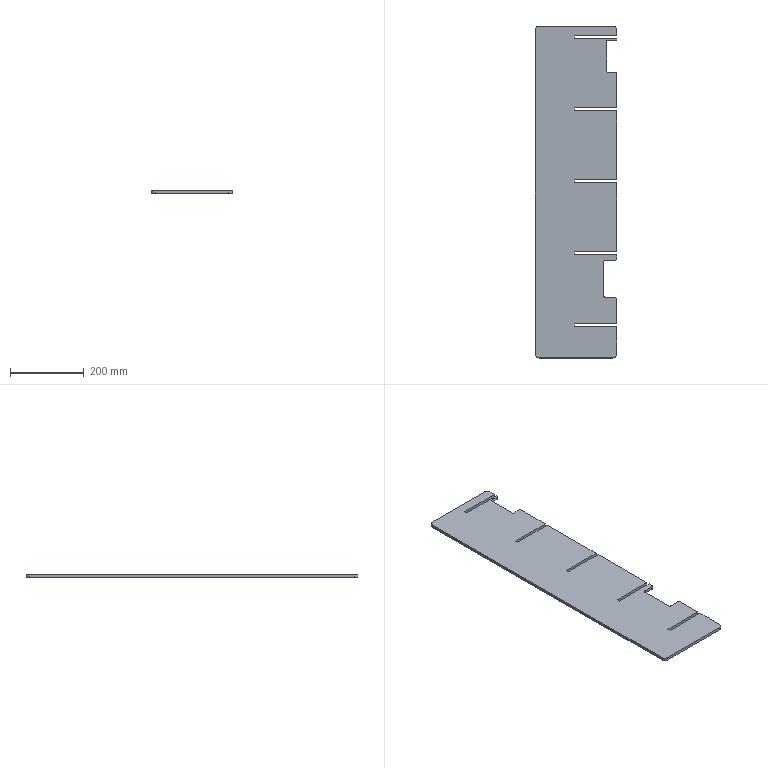Part | SolidWorks | features FlatPattern 1, SMBaseFlange 1, SheetMetal 1 | 1 solid | 46 faces | box 220 x 900 x 8 mm | volume 1500106 mm3 | plane 34 | cylinder 12 | commonest cylinder face diameters 4 x4 10 x4 20 x4
STEP:
#1=CARTESIAN_POINT('',(-1005.006,-530.938,0.));
#2=VERTEX_POINT('',#1);
#3=CARTESIAN_POINT('',(-995.006,-520.938,0.));
#4=VERTEX_POINT('',#3);
#5=CARTESIAN_POINT('',(-1005.006,-520.938,0.));
#6=DIRECTION('',(0.,0.,1.));
#7=DIRECTION('',(-1.,0.,0.));
#8=AXIS2_PLACEMENT_3D('',#5,#6,#7);
#9=CIRCLE('',#8,10.);
#10=EDGE_CURVE('',#2,#4,#9,.T.);
#11=ORIENTED_EDGE('',*,*,#10,.F.);
#12=CARTESIAN_POINT('',(-1005.006,-530.938,-8.));
#13=VERTEX_POINT('',#12);
#14=CARTESIAN_POINT('',(-1005.006,-530.938,-8.));
#15=DIRECTION('',(0.,0.,1.));
#16=VECTOR('',#15,1000.);
#17=LINE('',#14,#16);
#18=EDGE_CURVE('',#13,#2,#17,.T.);
#19=ORIENTED_EDGE('',*,*,#18,.F.);
#20=CARTESIAN_POINT('',(-995.006,-520.938,-8.));
#21=VERTEX_POINT('',#20);
#22=CARTESIAN_POINT('',(-1005.006,-520.938,-8.));
#23=DIRECTION('',(0.,0.,1.));
#24=DIRECTION('',(-1.,0.,0.));
#25=AXIS2_PLACEMENT_3D('',#22,#23,#24);
#26=CIRCLE('',#25,10.);
#27=EDGE_CURVE('',#13,#21,#26,.T.);
#28=ORIENTED_EDGE('',*,*,#27,.T.);
#29=CARTESIAN_POINT('',(-995.006,-520.938,-8.));
#30=DIRECTION('',(0.,0.,1.));
#31=VECTOR('',#30,1000.);
#32=LINE('',#29,#31);
#33=EDGE_CURVE('',#21,#4,#32,.T.);
#34=ORIENTED_EDGE('',*,*,#33,.T.);
#35=EDGE_LOOP('',(#11,#19,#28,#34));
#36=FACE_OUTER_BOUND('',#35,.T.);
#37=CARTESIAN_POINT('',(-1005.006,-520.938,-8.));
#38=DIRECTION('',(0.,0.,1.));
#39=DIRECTION('',(1.,0.,0.));
#40=AXIS2_PLACEMENT_3D('',#37,#38,#39);
#41=CYLINDRICAL_SURFACE('',#40,10.);
#42=ADVANCED_FACE('',(#36),#41,.T.);
#43=CARTESIAN_POINT('',(-1205.006,-530.938,0.));
#44=VERTEX_POINT('',#43);
#45=CARTESIAN_POINT('',(-1005.006,-530.938,0.));
#46=DIRECTION('',(1.,0.,0.));
#47=VECTOR('',#46,1000.);
#48=LINE('',#45,#47);
#49=EDGE_CURVE('',#44,#2,#48,.T.);
#50=ORIENTED_EDGE('',*,*,#49,.F.);
#51=CARTESIAN_POINT('',(-1205.006,-530.938,-8.));
#52=VERTEX_POINT('',#51);
#53=CARTESIAN_POINT('',(-1205.006,-530.938,-8.));
#54=DIRECTION('',(0.,0.,1.));
#55=VECTOR('',#54,1000.);
#56=LINE('',#53,#55);
#57=EDGE_CURVE('',#52,#44,#56,.T.);
#58=ORIENTED_EDGE('',*,*,#57,.F.);
#59=CARTESIAN_POINT('',(-1005.006,-530.938,-8.));
#60=DIRECTION('',(1.,0.,0.));
#61=VECTOR('',#60,1000.);
#62=LINE('',#59,#61);
#63=EDGE_CURVE('',#52,#13,#62,.T.);
#64=ORIENTED_EDGE('',*,*,#63,.T.);
#65=ORIENTED_EDGE('',*,*,#18,.T.);
#66=EDGE_LOOP('',(#50,#58,#64,#65));
#67=FACE_OUTER_BOUND('',#66,.T.);
#68=CARTESIAN_POINT('',(-1005.006,-530.938,-8.));
#69=DIRECTION('',(0.,-1.,0.));
#70=DIRECTION('',(1.,0.,0.));
#71=AXIS2_PLACEMENT_3D('',#68,#69,#70);
#72=PLANE('',#71);
#73=ADVANCED_FACE('',(#67),#72,.T.);
#74=CARTESIAN_POINT('',(-1215.006,-520.938,0.));
#75=VERTEX_POINT('',#74);
#76=CARTESIAN_POINT('',(-1205.006,-520.938,0.));
#77=DIRECTION('',(0.,0.,1.));
#78=DIRECTION('',(-1.,0.,0.));
#79=AXIS2_PLACEMENT_3D('',#76,#77,#78);
#80=CIRCLE('',#79,10.);
#81=EDGE_CURVE('',#75,#44,#80,.T.);
#82=ORIENTED_EDGE('',*,*,#81,.F.);
#83=CARTESIAN_POINT('',(-1215.006,-520.938,-8.));
#84=VERTEX_POINT('',#83);
#85=CARTESIAN_POINT('',(-1215.006,-520.938,-8.));
#86=DIRECTION('',(0.,0.,1.));
#87=VECTOR('',#86,1000.);
#88=LINE('',#85,#87);
#89=EDGE_CURVE('',#84,#75,#88,.T.);
#90=ORIENTED_EDGE('',*,*,#89,.F.);
#91=CARTESIAN_POINT('',(-1205.006,-520.938,-8.));
#92=DIRECTION('',(0.,0.,1.));
#93=DIRECTION('',(-1.,0.,0.));
#94=AXIS2_PLACEMENT_3D('',#91,#92,#93);
#95=CIRCLE('',#94,10.);
#96=EDGE_CURVE('',#84,#52,#95,.T.);
#97=ORIENTED_EDGE('',*,*,#96,.T.);
#98=ORIENTED_EDGE('',*,*,#57,.T.);
#99=EDGE_LOOP('',(#82,#90,#97,#98));
#100=FACE_OUTER_BOUND('',#99,.T.);
#101=CARTESIAN_POINT('',(-1205.006,-520.938,-8.));
#102=DIRECTION('',(0.,0.,1.));
#103=DIRECTION('',(1.,0.,0.));
#104=AXIS2_PLACEMENT_3D('',#101,#102,#103);
#105=CYLINDRICAL_SURFACE('',#104,10.);
#106=ADVANCED_FACE('',(#100),#105,.T.);
#107=CARTESIAN_POINT('',(-1215.006,359.062,0.));
#108=VERTEX_POINT('',#107);
#109=CARTESIAN_POINT('',(-1215.006,359.062,0.));
#110=DIRECTION('',(0.,-1.,0.));
#111=VECTOR('',#110,1000.);
#112=LINE('',#109,#111);
#113=EDGE_CURVE('',#108,#75,#112,.T.);
#114=ORIENTED_EDGE('',*,*,#113,.F.);
#115=CARTESIAN_POINT('',(-1215.006,359.062,-8.));
#116=VERTEX_POINT('',#115);
#117=CARTESIAN_POINT('',(-1215.006,359.062,-8.));
#118=DIRECTION('',(0.,0.,1.));
#119=VECTOR('',#118,1000.);
#120=LINE('',#117,#119);
#121=EDGE_CURVE('',#116,#108,#120,.T.);
#122=ORIENTED_EDGE('',*,*,#121,.F.);
#123=CARTESIAN_POINT('',(-1215.006,359.062,-8.));
#124=DIRECTION('',(0.,-1.,0.));
#125=VECTOR('',#124,1000.);
#126=LINE('',#123,#125);
#127=EDGE_CURVE('',#116,#84,#126,.T.);
#128=ORIENTED_EDGE('',*,*,#127,.T.);
#129=ORIENTED_EDGE('',*,*,#89,.T.);
#130=EDGE_LOOP('',(#114,#122,#128,#129));
#131=FACE_OUTER_BOUND('',#130,.T.);
#132=CARTESIAN_POINT('',(-1215.006,359.062,-8.));
#133=DIRECTION('',(-1.,0.,0.));
#134=DIRECTION('',(0.,0.,1.));
#135=AXIS2_PLACEMENT_3D('',#132,#133,#134);
#136=PLANE('',#135);
#137=ADVANCED_FACE('',(#131),#136,.T.);
#138=CARTESIAN_POINT('',(-1205.006,369.062,0.));
#139=VERTEX_POINT('',#138);
#140=CARTESIAN_POINT('',(-1205.006,359.062,0.));
#141=DIRECTION('',(0.,0.,1.));
#142=DIRECTION('',(1.,0.,0.));
#143=AXIS2_PLACEMENT_3D('',#140,#141,#142);
#144=CIRCLE('',#143,10.);
#145=EDGE_CURVE('',#139,#108,#144,.T.);
#146=ORIENTED_EDGE('',*,*,#145,.F.);
#147=CARTESIAN_POINT('',(-1205.006,369.062,-8.));
#148=VERTEX_POINT('',#147);
#149=CARTESIAN_POINT('',(-1205.006,369.062,-8.));
#150=DIRECTION('',(0.,0.,1.));
#151=VECTOR('',#150,1000.);
#152=LINE('',#149,#151);
#153=EDGE_CURVE('',#148,#139,#152,.T.);
#154=ORIENTED_EDGE('',*,*,#153,.F.);
#155=CARTESIAN_POINT('',(-1205.006,359.062,-8.));
#156=DIRECTION('',(0.,0.,1.));
#157=DIRECTION('',(1.,0.,0.));
#158=AXIS2_PLACEMENT_3D('',#155,#156,#157);
#159=CIRCLE('',#158,10.);
#160=EDGE_CURVE('',#148,#116,#159,.T.);
#161=ORIENTED_EDGE('',*,*,#160,.T.);
#162=ORIENTED_EDGE('',*,*,#121,.T.);
#163=EDGE_LOOP('',(#146,#154,#161,#162));
#164=FACE_OUTER_BOUND('',#163,.T.);
#165=CARTESIAN_POINT('',(-1205.006,359.062,-8.));
#166=DIRECTION('',(0.,0.,1.));
#167=DIRECTION('',(1.,0.,0.));
#168=AXIS2_PLACEMENT_3D('',#165,#166,#167);
#169=CYLINDRICAL_SURFACE('',#168,10.);
#170=ADVANCED_FACE('',(#164),#169,.T.);
#171=CARTESIAN_POINT('',(-1005.006,369.062,0.));
#172=VERTEX_POINT('',#171);
#173=CARTESIAN_POINT('',(-1005.006,369.062,0.));
#174=DIRECTION('',(-1.,0.,0.));
#175=VECTOR('',#174,1000.);
#176=LINE('',#173,#175);
#177=EDGE_CURVE('',#172,#139,#176,.T.);
#178=ORIENTED_EDGE('',*,*,#177,.F.);
#179=CARTESIAN_POINT('',(-1005.006,369.062,-8.));
#180=VERTEX_POINT('',#179);
#181=CARTESIAN_POINT('',(-1005.006,369.062,-8.));
#182=DIRECTION('',(0.,0.,1.));
#183=VECTOR('',#182,1000.);
#184=LINE('',#181,#183);
#185=EDGE_CURVE('',#180,#172,#184,.T.);
#186=ORIENTED_EDGE('',*,*,#185,.F.);
#187=CARTESIAN_POINT('',(-1005.006,369.062,-8.));
#188=DIRECTION('',(-1.,0.,0.));
#189=VECTOR('',#188,1000.);
#190=LINE('',#187,#189);
#191=EDGE_CURVE('',#180,#148,#190,.T.);
#192=ORIENTED_EDGE('',*,*,#191,.T.);
#193=ORIENTED_EDGE('',*,*,#153,.T.);
#194=EDGE_LOOP('',(#178,#186,#192,#193));
#195=FACE_OUTER_BOUND('',#194,.T.);
#196=CARTESIAN_POINT('',(-1005.006,369.062,-8.));
#197=DIRECTION('',(0.,1.,0.));
#198=DIRECTION('',(0.,0.,1.));
#199=AXIS2_PLACEMENT_3D('',#196,#197,#198);
#200=PLANE('',#199);
#201=ADVANCED_FACE('',(#195),#200,.T.);
#202=CARTESIAN_POINT('',(-995.006,359.062,0.));
#203=VERTEX_POINT('',#202);
#204=CARTESIAN_POINT('',(-1005.006,359.062,0.));
#205=DIRECTION('',(0.,0.,1.));
#206=DIRECTION('',(-1.,0.,0.));
#207=AXIS2_PLACEMENT_3D('',#204,#205,#206);
#208=CIRCLE('',#207,10.);
#209=EDGE_CURVE('',#203,#172,#208,.T.);
#210=ORIENTED_EDGE('',*,*,#209,.F.);
#211=CARTESIAN_POINT('',(-995.006,359.062,-8.));
#212=VERTEX_POINT('',#211);
#213=CARTESIAN_POINT('',(-995.006,359.062,-8.));
#214=DIRECTION('',(0.,0.,1.));
#215=VECTOR('',#214,1000.);
#216=LINE('',#213,#215);
#217=EDGE_CURVE('',#212,#203,#216,.T.);
#218=ORIENTED_EDGE('',*,*,#217,.F.);
#219=CARTESIAN_POINT('',(-1005.006,359.062,-8.));
#220=DIRECTION('',(0.,0.,1.));
#221=DIRECTION('',(-1.,0.,0.));
#222=AXIS2_PLACEMENT_3D('',#219,#220,#221);
#223=CIRCLE('',#222,10.);
#224=EDGE_CURVE('',#212,#180,#223,.T.);
#225=ORIENTED_EDGE('',*,*,#224,.T.);
#226=ORIENTED_EDGE('',*,*,#185,.T.);
#227=EDGE_LOOP('',(#210,#218,#225,#226));
#228=FACE_OUTER_BOUND('',#227,.T.);
#229=CARTESIAN_POINT('',(-1005.006,359.062,-8.));
#230=DIRECTION('',(0.,0.,1.));
#231=DIRECTION('',(1.,0.,0.));
#232=AXIS2_PLACEMENT_3D('',#229,#230,#231);
#233=CYLINDRICAL_SURFACE('',#232,10.);
#234=ADVANCED_FACE('',(#228),#233,.T.);
#235=CARTESIAN_POINT('',(-995.006,342.062,0.));
#236=VERTEX_POINT('',#235);
#237=CARTESIAN_POINT('',(-995.006,359.062,0.));
#238=DIRECTION('',(0.,1.,0.));
#239=VECTOR('',#238,1000.);
#240=LINE('',#237,#239);
#241=EDGE_CURVE('',#236,#203,#240,.T.);
#242=ORIENTED_EDGE('',*,*,#241,.F.);
#243=CARTESIAN_POINT('',(-995.006,342.062,-8.));
#244=VERTEX_POINT('',#243);
#245=CARTESIAN_POINT('',(-995.006,342.062,-8.));
#246=DIRECTION('',(0.,0.,1.));
#247=VECTOR('',#246,1000.);
#248=LINE('',#245,#247);
#249=EDGE_CURVE('',#244,#236,#248,.T.);
#250=ORIENTED_EDGE('',*,*,#249,.F.);
#251=CARTESIAN_POINT('',(-995.006,359.062,-8.));
#252=DIRECTION('',(0.,1.,0.));
#253=VECTOR('',#252,1000.);
#254=LINE('',#251,#253);
#255=EDGE_CURVE('',#244,#212,#254,.T.);
#256=ORIENTED_EDGE('',*,*,#255,.T.);
#257=ORIENTED_EDGE('',*,*,#217,.T.);
#258=EDGE_LOOP('',(#242,#250,#256,#257));
#259=FACE_OUTER_BOUND('',#258,.T.);
#260=CARTESIAN_POINT('',(-995.006,359.062,-8.));
#261=DIRECTION('',(1.,0.,0.));
#262=DIRECTION('',(0.,0.,-1.));
#263=AXIS2_PLACEMENT_3D('',#260,#261,#262);
#264=PLANE('',#263);
#265=ADVANCED_FACE('',(#259),#264,.T.);
#266=CARTESIAN_POINT('',(-1109.506,342.062,0.));
#267=VERTEX_POINT('',#266);
#268=CARTESIAN_POINT('',(-995.006,342.062,0.));
#269=DIRECTION('',(1.,0.,0.));
#270=VECTOR('',#269,1000.);
#271=LINE('',#268,#270);
#272=EDGE_CURVE('',#267,#236,#271,.T.);
#273=ORIENTED_EDGE('',*,*,#272,.F.);
#274=CARTESIAN_POINT('',(-1109.506,342.062,-8.));
#275=VERTEX_POINT('',#274);
#276=CARTESIAN_POINT('',(-1109.506,342.062,-8.));
#277=DIRECTION('',(0.,0.,1.));
#278=VECTOR('',#277,1000.);
#279=LINE('',#276,#278);
#280=EDGE_CURVE('',#275,#267,#279,.T.);
#281=ORIENTED_EDGE('',*,*,#280,.F.);
#282=CARTESIAN_POINT('',(-995.006,342.062,-8.));
#283=DIRECTION('',(1.,0.,0.));
#284=VECTOR('',#283,1000.);
#285=LINE('',#282,#284);
#286=EDGE_CURVE('',#275,#244,#285,.T.);
#287=ORIENTED_EDGE('',*,*,#286,.T.);
#288=ORIENTED_EDGE('',*,*,#249,.T.);
#289=EDGE_LOOP('',(#273,#281,#287,#288));
#290=FACE_OUTER_BOUND('',#289,.T.);
#291=CARTESIAN_POINT('',(-995.006,342.062,-8.));
#292=DIRECTION('',(0.,-1.,0.));
#293=DIRECTION('',(0.,0.,-1.));
#294=AXIS2_PLACEMENT_3D('',#291,#292,#293);
#295=PLANE('',#294);
#296=ADVANCED_FACE('',(#290),#295,.T.);
#297=CARTESIAN_POINT('',(-1109.506,334.062,0.));
#298=VERTEX_POINT('',#297);
#299=CARTESIAN_POINT('',(-1109.506,342.062,0.));
#300=DIRECTION('',(0.,1.,0.));
#301=VECTOR('',#300,1000.);
#302=LINE('',#299,#301);
#303=EDGE_CURVE('',#298,#267,#302,.T.);
#304=ORIENTED_EDGE('',*,*,#303,.F.);
#305=CARTESIAN_POINT('',(-1109.506,334.062,-8.));
#306=VERTEX_POINT('',#305);
#307=CARTESIAN_POINT('',(-1109.506,334.062,-8.));
#308=DIRECTION('',(0.,0.,1.));
#309=VECTOR('',#308,1000.);
#310=LINE('',#307,#309);
#311=EDGE_CURVE('',#306,#298,#310,.T.);
#312=ORIENTED_EDGE('',*,*,#311,.F.);
#313=CARTESIAN_POINT('',(-1109.506,342.062,-8.));
#314=DIRECTION('',(0.,1.,0.));
#315=VECTOR('',#314,1000.);
#316=LINE('',#313,#315);
#317=EDGE_CURVE('',#306,#275,#316,.T.);
#318=ORIENTED_EDGE('',*,*,#317,.T.);
#319=ORIENTED_EDGE('',*,*,#280,.T.);
#320=EDGE_LOOP('',(#304,#312,#318,#319));
#321=FACE_OUTER_BOUND('',#320,.T.);
#322=CARTESIAN_POINT('',(-1109.506,342.062,-8.));
#323=DIRECTION('',(1.,0.,0.));
#324=DIRECTION('',(0.,0.,-1.));
#325=AXIS2_PLACEMENT_3D('',#322,#323,#324);
#326=PLANE('',#325);
#327=ADVANCED_FACE('',(#321),#326,.T.);
#328=CARTESIAN_POINT('',(-995.006,334.062,0.));
#329=VERTEX_POINT('',#328);
#330=CARTESIAN_POINT('',(-1109.506,334.062,0.));
#331=DIRECTION('',(-1.,0.,0.));
#332=VECTOR('',#331,1000.);
#333=LINE('',#330,#332);
#334=EDGE_CURVE('',#329,#298,#333,.T.);
#335=ORIENTED_EDGE('',*,*,#334,.F.);
#336=CARTESIAN_POINT('',(-995.006,334.062,-8.));
#337=VERTEX_POINT('',#336);
#338=CARTESIAN_POINT('',(-995.006,334.062,-8.));
#339=DIRECTION('',(0.,0.,1.));
#340=VECTOR('',#339,1000.);
#341=LINE('',#338,#340);
#342=EDGE_CURVE('',#337,#329,#341,.T.);
#343=ORIENTED_EDGE('',*,*,#342,.F.);
#344=CARTESIAN_POINT('',(-1109.506,334.062,-8.));
#345=DIRECTION('',(-1.,0.,0.));
#346=VECTOR('',#345,1000.);
#347=LINE('',#344,#346);
#348=EDGE_CURVE('',#337,#306,#347,.T.);
#349=ORIENTED_EDGE('',*,*,#348,.T.);
#350=ORIENTED_EDGE('',*,*,#311,.T.);
#351=EDGE_LOOP('',(#335,#343,#349,#350));
#352=FACE_OUTER_BOUND('',#351,.T.);
#353=CARTESIAN_POINT('',(-1109.506,334.062,-8.));
#354=DIRECTION('',(0.,1.,0.));
#355=DIRECTION('',(0.,0.,1.));
#356=AXIS2_PLACEMENT_3D('',#353,#354,#355);
#357=PLANE('',#356);
#358=ADVANCED_FACE('',(#352),#357,.T.);
#359=CARTESIAN_POINT('',(-995.006,331.062,0.));
#360=VERTEX_POINT('',#359);
#361=CARTESIAN_POINT('',(-995.006,334.062,0.));
#362=DIRECTION('',(0.,1.,0.));
#363=VECTOR('',#362,1000.);
#364=LINE('',#361,#363);
#365=EDGE_CURVE('',#360,#329,#364,.T.);
#366=ORIENTED_EDGE('',*,*,#365,.F.);
#367=CARTESIAN_POINT('',(-995.006,331.062,-8.));
#368=VERTEX_POINT('',#367);
#369=CARTESIAN_POINT('',(-995.006,331.062,-8.));
#370=DIRECTION('',(0.,0.,1.));
#371=VECTOR('',#370,1000.);
#372=LINE('',#369,#371);
#373=EDGE_CURVE('',#368,#360,#372,.T.);
#374=ORIENTED_EDGE('',*,*,#373,.F.);
#375=CARTESIAN_POINT('',(-995.006,334.062,-8.));
#376=DIRECTION('',(0.,1.,0.));
#377=VECTOR('',#376,1000.);
#378=LINE('',#375,#377);
#379=EDGE_CURVE('',#368,#337,#378,.T.);
#380=ORIENTED_EDGE('',*,*,#379,.T.);
#381=ORIENTED_EDGE('',*,*,#342,.T.);
#382=EDGE_LOOP('',(#366,#374,#380,#381));
#383=FACE_OUTER_BOUND('',#382,.T.);
#384=CARTESIAN_POINT('',(-995.006,334.062,-8.));
#385=DIRECTION('',(1.,0.,0.));
#386=DIRECTION('',(0.,0.,-1.));
#387=AXIS2_PLACEMENT_3D('',#384,#385,#386);
#388=PLANE('',#387);
#389=ADVANCED_FACE('',(#383),#388,.T.);
#390=CARTESIAN_POINT('',(-997.006,329.062,0.));
#391=VERTEX_POINT('',#390);
#392=CARTESIAN_POINT('',(-997.006,331.062,0.));
#393=DIRECTION('',(0.,0.,1.));
#394=DIRECTION('',(1.,0.,0.));
#395=AXIS2_PLACEMENT_3D('',#392,#393,#394);
#396=CIRCLE('',#395,2.);
#397=EDGE_CURVE('',#391,#360,#396,.T.);
#398=ORIENTED_EDGE('',*,*,#397,.F.);
#399=CARTESIAN_POINT('',(-997.006,329.062,-8.));
#400=VERTEX_POINT('',#399);
#401=CARTESIAN_POINT('',(-997.006,329.062,-8.));
#402=DIRECTION('',(0.,0.,1.));
#403=VECTOR('',#402,1000.);
#404=LINE('',#401,#403);
#405=EDGE_CURVE('',#400,#391,#404,.T.);
#406=ORIENTED_EDGE('',*,*,#405,.F.);
#407=CARTESIAN_POINT('',(-997.006,331.062,-8.));
#408=DIRECTION('',(0.,0.,1.));
#409=DIRECTION('',(1.,0.,0.));
#410=AXIS2_PLACEMENT_3D('',#407,#408,#409);
#411=CIRCLE('',#410,2.);
#412=EDGE_CURVE('',#400,#368,#411,.T.);
#413=ORIENTED_EDGE('',*,*,#412,.T.);
#414=ORIENTED_EDGE('',*,*,#373,.T.);
#415=EDGE_LOOP('',(#398,#406,#413,#414));
#416=FACE_OUTER_BOUND('',#415,.T.);
#417=CARTESIAN_POINT('',(-997.006,331.062,-8.));
#418=DIRECTION('',(0.,0.,1.));
#419=DIRECTION('',(1.,0.,0.));
#420=AXIS2_PLACEMENT_3D('',#417,#418,#419);
#421=CYLINDRICAL_SURFACE('',#420,2.);
#422=ADVANCED_FACE('',(#416),#421,.T.);
#423=CARTESIAN_POINT('',(-1019.723,329.062,0.));
#424=VERTEX_POINT('',#423);
#425=CARTESIAN_POINT('',(-1019.723,329.062,0.));
#426=DIRECTION('',(1.,0.,0.));
#427=VECTOR('',#426,1000.);
#428=LINE('',#425,#427);
#429=EDGE_CURVE('',#424,#391,#428,.T.);
#430=ORIENTED_EDGE('',*,*,#429,.F.);
#431=CARTESIAN_POINT('',(-1019.723,329.062,-8.));
#432=VERTEX_POINT('',#431);
#433=CARTESIAN_POINT('',(-1019.723,329.062,-8.));
#434=DIRECTION('',(0.,0.,1.));
#435=VECTOR('',#434,1000.);
#436=LINE('',#433,#435);
#437=EDGE_CURVE('',#432,#424,#436,.T.);
#438=ORIENTED_EDGE('',*,*,#437,.F.);
#439=CARTESIAN_POINT('',(-1019.723,329.062,-8.));
#440=DIRECTION('',(1.,0.,0.));
#441=VECTOR('',#440,1000.);
#442=LINE('',#439,#441);
#443=EDGE_CURVE('',#432,#400,#442,.T.);
#444=ORIENTED_EDGE('',*,*,#443,.T.);
#445=ORIENTED_EDGE('',*,*,#405,.T.);
#446=EDGE_LOOP('',(#430,#438,#444,#445));
#447=FACE_OUTER_BOUND('',#446,.T.);
#448=CARTESIAN_POINT('',(-1019.723,329.062,-8.));
#449=DIRECTION('',(0.,-1.,0.));
#450=DIRECTION('',(0.,0.,-1.));
#451=AXIS2_PLACEMENT_3D('',#448,#449,#450);
#452=PLANE('',#451);
#453=ADVANCED_FACE('',(#447),#452,.T.);
#454=CARTESIAN_POINT('',(-1021.723,327.062,0.));
#455=VERTEX_POINT('',#454);
#456=CARTESIAN_POINT('',(-1019.723,327.062,0.));
#457=DIRECTION('',(0.,0.,-1.));
#458=DIRECTION('',(-1.,0.,0.));
#459=AXIS2_PLACEMENT_3D('',#456,#457,#458);
#460=CIRCLE('',#459,2.);
#461=EDGE_CURVE('',#455,#424,#460,.T.);
#462=ORIENTED_EDGE('',*,*,#461,.F.);
#463=CARTESIAN_POINT('',(-1021.723,327.062,-8.));
#464=VERTEX_POINT('',#463);
#465=CARTESIAN_POINT('',(-1021.723,327.062,-8.));
#466=DIRECTION('',(0.,0.,1.));
#467=VECTOR('',#466,1000.);
#468=LINE('',#465,#467);
#469=EDGE_CURVE('',#464,#455,#468,.T.);
#470=ORIENTED_EDGE('',*,*,#469,.F.);
#471=CARTESIAN_POINT('',(-1019.723,327.062,-8.));
#472=DIRECTION('',(0.,0.,-1.));
#473=DIRECTION('',(-1.,0.,0.));
#474=AXIS2_PLACEMENT_3D('',#471,#472,#473);
#475=CIRCLE('',#474,2.);
#476=EDGE_CURVE('',#464,#432,#475,.T.);
#477=ORIENTED_EDGE('',*,*,#476,.T.);
#478=ORIENTED_EDGE('',*,*,#437,.T.);
#479=EDGE_LOOP('',(#462,#470,#477,#478));
#480=FACE_OUTER_BOUND('',#479,.T.);
#481=CARTESIAN_POINT('',(-1019.723,327.062,-8.));
#482=DIRECTION('',(0.,0.,1.));
#483=DIRECTION('',(1.,0.,0.));
#484=AXIS2_PLACEMENT_3D('',#481,#482,#483);
#485=CYLINDRICAL_SURFACE('',#484,2.);
#486=ADVANCED_FACE('',(#480),#485,.F.);
#487=CARTESIAN_POINT('',(-1021.723,246.062,0.));
#488=VERTEX_POINT('',#487);
#489=CARTESIAN_POINT('',(-1021.723,246.062,0.));
#490=DIRECTION('',(0.,1.,0.));
#491=VECTOR('',#490,1000.);
#492=LINE('',#489,#491);
#493=EDGE_CURVE('',#488,#455,#492,.T.);
#494=ORIENTED_EDGE('',*,*,#493,.F.);
#495=CARTESIAN_POINT('',(-1021.723,246.062,-8.));
#496=VERTEX_POINT('',#495);
#497=CARTESIAN_POINT('',(-1021.723,246.062,-8.));
#498=DIRECTION('',(0.,0.,1.));
#499=VECTOR('',#498,1000.);
#500=LINE('',#497,#499);
#501=EDGE_CURVE('',#496,#488,#500,.T.);
#502=ORIENTED_EDGE('',*,*,#501,.F.);
#503=CARTESIAN_POINT('',(-1021.723,246.062,-8.));
#504=DIRECTION('',(0.,1.,0.));
#505=VECTOR('',#504,1000.);
#506=LINE('',#503,#505);
#507=EDGE_CURVE('',#496,#464,#506,.T.);
#508=ORIENTED_EDGE('',*,*,#507,.T.);
#509=ORIENTED_EDGE('',*,*,#469,.T.);
#510=EDGE_LOOP('',(#494,#502,#508,#509));
#511=FACE_OUTER_BOUND('',#510,.T.);
#512=CARTESIAN_POINT('',(-1021.723,246.062,-8.));
#513=DIRECTION('',(1.,0.,0.));
#514=DIRECTION('',(0.,0.,-1.));
#515=AXIS2_PLACEMENT_3D('',#512,#513,#514);
#516=PLANE('',#515);
#517=ADVANCED_FACE('',(#511),#516,.T.);
#518=CARTESIAN_POINT('',(-1019.723,244.062,0.));
#519=VERTEX_POINT('',#518);
#520=CARTESIAN_POINT('',(-1019.723,246.062,0.));
#521=DIRECTION('',(0.,0.,-1.));
#522=DIRECTION('',(-1.,0.,0.));
#523=AXIS2_PLACEMENT_3D('',#520,#521,#522);
#524=CIRCLE('',#523,2.);
#525=EDGE_CURVE('',#519,#488,#524,.T.);
#526=ORIENTED_EDGE('',*,*,#525,.F.);
#527=CARTESIAN_POINT('',(-1019.723,244.062,-8.));
#528=VERTEX_POINT('',#527);
#529=CARTESIAN_POINT('',(-1019.723,244.062,-8.));
#530=DIRECTION('',(0.,0.,1.));
#531=VECTOR('',#530,1000.);
#532=LINE('',#529,#531);
#533=EDGE_CURVE('',#528,#519,#532,.T.);
#534=ORIENTED_EDGE('',*,*,#533,.F.);
#535=CARTESIAN_POINT('',(-1019.723,246.062,-8.));
#536=DIRECTION('',(0.,0.,-1.));
#537=DIRECTION('',(-1.,0.,0.));
#538=AXIS2_PLACEMENT_3D('',#535,#536,#537);
#539=CIRCLE('',#538,2.);
#540=EDGE_CURVE('',#528,#496,#539,.T.);
#541=ORIENTED_EDGE('',*,*,#540,.T.);
#542=ORIENTED_EDGE('',*,*,#501,.T.);
#543=EDGE_LOOP('',(#526,#534,#541,#542));
#544=FACE_OUTER_BOUND('',#543,.T.);
#545=CARTESIAN_POINT('',(-1019.723,246.062,-8.));
#546=DIRECTION('',(0.,0.,1.));
#547=DIRECTION('',(1.,0.,0.));
#548=AXIS2_PLACEMENT_3D('',#545,#546,#547);
#549=CYLINDRICAL_SURFACE('',#548,2.);
#550=ADVANCED_FACE('',(#544),#549,.F.);
#551=CARTESIAN_POINT('',(-997.006,244.062,0.));
#552=VERTEX_POINT('',#551);
#553=CARTESIAN_POINT('',(-997.006,244.062,0.));
#554=DIRECTION('',(-1.,0.,0.));
#555=VECTOR('',#554,1000.);
#556=LINE('',#553,#555);
#557=EDGE_CURVE('',#552,#519,#556,.T.);
#558=ORIENTED_EDGE('',*,*,#557,.F.);
#559=CARTESIAN_POINT('',(-997.006,244.062,-8.));
#560=VERTEX_POINT('',#559);
#561=CARTESIAN_POINT('',(-997.006,244.062,-8.));
#562=DIRECTION('',(0.,0.,1.));
#563=VECTOR('',#562,1000.);
#564=LINE('',#561,#563);
#565=EDGE_CURVE('',#560,#552,#564,.T.);
#566=ORIENTED_EDGE('',*,*,#565,.F.);
#567=CARTESIAN_POINT('',(-997.006,244.062,-8.));
#568=DIRECTION('',(-1.,0.,0.));
#569=VECTOR('',#568,1000.);
#570=LINE('',#567,#569);
#571=EDGE_CURVE('',#560,#528,#570,.T.);
#572=ORIENTED_EDGE('',*,*,#571,.T.);
#573=ORIENTED_EDGE('',*,*,#533,.T.);
#574=EDGE_LOOP('',(#558,#566,#572,#573));
#575=FACE_OUTER_BOUND('',#574,.T.);
#576=CARTESIAN_POINT('',(-997.006,244.062,-8.));
#577=DIRECTION('',(0.,1.,0.));
#578=DIRECTION('',(-1.,0.,0.));
#579=AXIS2_PLACEMENT_3D('',#576,#577,#578);
#580=PLANE('',#579);
#581=ADVANCED_FACE('',(#575),#580,.T.);
#582=CARTESIAN_POINT('',(-995.006,242.062,0.));
#583=VERTEX_POINT('',#582);
#584=CARTESIAN_POINT('',(-997.006,242.062,0.));
#585=DIRECTION('',(0.,0.,1.));
#586=DIRECTION('',(-1.,0.,0.));
#587=AXIS2_PLACEMENT_3D('',#584,#585,#586);
#588=CIRCLE('',#587,2.);
#589=EDGE_CURVE('',#583,#552,#588,.T.);
#590=ORIENTED_EDGE('',*,*,#589,.F.);
#591=CARTESIAN_POINT('',(-995.006,242.062,-8.));
#592=VERTEX_POINT('',#591);
#593=CARTESIAN_POINT('',(-995.006,242.062,-8.));
#594=DIRECTION('',(0.,0.,1.));
#595=VECTOR('',#594,1000.);
#596=LINE('',#593,#595);
#597=EDGE_CURVE('',#592,#583,#596,.T.);
#598=ORIENTED_EDGE('',*,*,#597,.F.);
#599=CARTESIAN_POINT('',(-997.006,242.062,-8.));
#600=DIRECTION('',(0.,0.,1.));
#601=DIRECTION('',(-1.,0.,0.));
#602=AXIS2_PLACEMENT_3D('',#599,#600,#601);
#603=CIRCLE('',#602,2.);
#604=EDGE_CURVE('',#592,#560,#603,.T.);
#605=ORIENTED_EDGE('',*,*,#604,.T.);
#606=ORIENTED_EDGE('',*,*,#565,.T.);
#607=EDGE_LOOP('',(#590,#598,#605,#606));
#608=FACE_OUTER_BOUND('',#607,.T.);
#609=CARTESIAN_POINT('',(-997.006,242.062,-8.));
#610=DIRECTION('',(0.,0.,1.));
#611=DIRECTION('',(1.,0.,0.));
#612=AXIS2_PLACEMENT_3D('',#609,#610,#611);
#613=CYLINDRICAL_SURFACE('',#612,2.);
#614=ADVANCED_FACE('',(#608),#613,.T.);
#615=CARTESIAN_POINT('',(-995.006,147.062,0.));
#616=VERTEX_POINT('',#615);
#617=CARTESIAN_POINT('',(-995.006,242.062,0.));
#618=DIRECTION('',(0.,1.,0.));
#619=VECTOR('',#618,1000.);
#620=LINE('',#617,#619);
#621=EDGE_CURVE('',#616,#583,#620,.T.);
#622=ORIENTED_EDGE('',*,*,#621,.F.);
#623=CARTESIAN_POINT('',(-995.006,147.062,-8.));
#624=VERTEX_POINT('',#623);
#625=CARTESIAN_POINT('',(-995.006,147.062,-8.));
#626=DIRECTION('',(0.,0.,1.));
#627=VECTOR('',#626,1000.);
#628=LINE('',#625,#627);
#629=EDGE_CURVE('',#624,#616,#628,.T.);
#630=ORIENTED_EDGE('',*,*,#629,.F.);
#631=CARTESIAN_POINT('',(-995.006,242.062,-8.));
#632=DIRECTION('',(0.,1.,0.));
#633=VECTOR('',#632,1000.);
#634=LINE('',#631,#633);
#635=EDGE_CURVE('',#624,#592,#634,.T.);
#636=ORIENTED_EDGE('',*,*,#635,.T.);
#637=ORIENTED_EDGE('',*,*,#597,.T.);
#638=EDGE_LOOP('',(#622,#630,#636,#637));
#639=FACE_OUTER_BOUND('',#638,.T.);
#640=CARTESIAN_POINT('',(-995.006,242.062,-8.));
#641=DIRECTION('',(1.,0.,0.));
#642=DIRECTION('',(0.,1.,0.));
#643=AXIS2_PLACEMENT_3D('',#640,#641,#642);
#644=PLANE('',#643);
#645=ADVANCED_FACE('',(#639),#644,.T.);
#646=CARTESIAN_POINT('',(-1109.506,147.062,0.));
#647=VERTEX_POINT('',#646);
#648=CARTESIAN_POINT('',(-995.006,147.062,0.));
#649=DIRECTION('',(1.,0.,0.));
#650=VECTOR('',#649,1000.);
#651=LINE('',#648,#650);
#652=EDGE_CURVE('',#647,#616,#651,.T.);
#653=ORIENTED_EDGE('',*,*,#652,.F.);
#654=CARTESIAN_POINT('',(-1109.506,147.062,-8.));
#655=VERTEX_POINT('',#654);
#656=CARTESIAN_POINT('',(-1109.506,147.062,-8.));
#657=DIRECTION('',(0.,0.,1.));
#658=VECTOR('',#657,1000.);
#659=LINE('',#656,#658);
#660=EDGE_CURVE('',#655,#647,#659,.T.);
#661=ORIENTED_EDGE('',*,*,#660,.F.);
#662=CARTESIAN_POINT('',(-995.006,147.062,-8.));
#663=DIRECTION('',(1.,0.,0.));
#664=VECTOR('',#663,1000.);
#665=LINE('',#662,#664);
#666=EDGE_CURVE('',#655,#624,#665,.T.);
#667=ORIENTED_EDGE('',*,*,#666,.T.);
#668=ORIENTED_EDGE('',*,*,#629,.T.);
#669=EDGE_LOOP('',(#653,#661,#667,#668));
#670=FACE_OUTER_BOUND('',#669,.T.);
#671=CARTESIAN_POINT('',(-995.006,147.062,-8.));
#672=DIRECTION('',(0.,-1.,0.));
#673=DIRECTION('',(0.,0.,-1.));
#674=AXIS2_PLACEMENT_3D('',#671,#672,#673);
#675=PLANE('',#674);
#676=ADVANCED_FACE('',(#670),#675,.T.);
#677=CARTESIAN_POINT('',(-1109.506,139.062,0.));
#678=VERTEX_POINT('',#677);
#679=CARTESIAN_POINT('',(-1109.506,147.062,0.));
#680=DIRECTION('',(0.,1.,0.));
#681=VECTOR('',#680,1000.);
#682=LINE('',#679,#681);
#683=EDGE_CURVE('',#678,#647,#682,.T.);
#684=ORIENTED_EDGE('',*,*,#683,.F.);
#685=CARTESIAN_POINT('',(-1109.506,139.062,-8.));
#686=VERTEX_POINT('',#685);
#687=CARTESIAN_POINT('',(-1109.506,139.062,-8.));
#688=DIRECTION('',(0.,0.,1.));
#689=VECTOR('',#688,1000.);
#690=LINE('',#687,#689);
#691=EDGE_CURVE('',#686,#678,#690,.T.);
#692=ORIENTED_EDGE('',*,*,#691,.F.);
#693=CARTESIAN_POINT('',(-1109.506,147.062,-8.));
#694=DIRECTION('',(0.,1.,0.));
#695=VECTOR('',#694,1000.);
#696=LINE('',#693,#695);
#697=EDGE_CURVE('',#686,#655,#696,.T.);
#698=ORIENTED_EDGE('',*,*,#697,.T.);
#699=ORIENTED_EDGE('',*,*,#660,.T.);
#700=EDGE_LOOP('',(#684,#692,#698,#699));
#701=FACE_OUTER_BOUND('',#700,.T.);
#702=CARTESIAN_POINT('',(-1109.506,147.062,-8.));
#703=DIRECTION('',(1.,0.,0.));
#704=DIRECTION('',(0.,0.,-1.));
#705=AXIS2_PLACEMENT_3D('',#702,#703,#704);
#706=PLANE('',#705);
#707=ADVANCED_FACE('',(#701),#706,.T.);
#708=CARTESIAN_POINT('',(-995.006,139.062,0.));
#709=VERTEX_POINT('',#708);
#710=CARTESIAN_POINT('',(-1109.506,139.062,0.));
#711=DIRECTION('',(-1.,0.,0.));
#712=VECTOR('',#711,1000.);
#713=LINE('',#710,#712);
#714=EDGE_CURVE('',#709,#678,#713,.T.);
#715=ORIENTED_EDGE('',*,*,#714,.F.);
#716=CARTESIAN_POINT('',(-995.006,139.062,-8.));
#717=VERTEX_POINT('',#716);
#718=CARTESIAN_POINT('',(-995.006,139.062,-8.));
#719=DIRECTION('',(0.,0.,1.));
#720=VECTOR('',#719,1000.);
#721=LINE('',#718,#720);
#722=EDGE_CURVE('',#717,#709,#721,.T.);
#723=ORIENTED_EDGE('',*,*,#722,.F.);
#724=CARTESIAN_POINT('',(-1109.506,139.062,-8.));
#725=DIRECTION('',(-1.,0.,0.));
#726=VECTOR('',#725,1000.);
#727=LINE('',#724,#726);
#728=EDGE_CURVE('',#717,#686,#727,.T.);
#729=ORIENTED_EDGE('',*,*,#728,.T.);
#730=ORIENTED_EDGE('',*,*,#691,.T.);
#731=EDGE_LOOP('',(#715,#723,#729,#730));
#732=FACE_OUTER_BOUND('',#731,.T.);
#733=CARTESIAN_POINT('',(-1109.506,139.062,-8.));
#734=DIRECTION('',(0.,1.,0.));
#735=DIRECTION('',(0.,0.,1.));
#736=AXIS2_PLACEMENT_3D('',#733,#734,#735);
#737=PLANE('',#736);
#738=ADVANCED_FACE('',(#732),#737,.T.);
#739=CARTESIAN_POINT('',(-995.006,-47.938,0.));
#740=VERTEX_POINT('',#739);
#741=CARTESIAN_POINT('',(-995.006,139.062,0.));
#742=DIRECTION('',(0.,1.,0.));
#743=VECTOR('',#742,1000.);
#744=LINE('',#741,#743);
#745=EDGE_CURVE('',#740,#709,#744,.T.);
#746=ORIENTED_EDGE('',*,*,#745,.F.);
#747=CARTESIAN_POINT('',(-995.006,-47.938,-8.));
#748=VERTEX_POINT('',#747);
#749=CARTESIAN_POINT('',(-995.006,-47.938,-8.));
#750=DIRECTION('',(0.,0.,1.));
#751=VECTOR('',#750,1000.);
#752=LINE('',#749,#751);
#753=EDGE_CURVE('',#748,#740,#752,.T.);
#754=ORIENTED_EDGE('',*,*,#753,.F.);
#755=CARTESIAN_POINT('',(-995.006,139.062,-8.));
#756=DIRECTION('',(0.,1.,0.));
#757=VECTOR('',#756,1000.);
#758=LINE('',#755,#757);
#759=EDGE_CURVE('',#748,#717,#758,.T.);
#760=ORIENTED_EDGE('',*,*,#759,.T.);
#761=ORIENTED_EDGE('',*,*,#722,.T.);
#762=EDGE_LOOP('',(#746,#754,#760,#761));
#763=FACE_OUTER_BOUND('',#762,.T.);
#764=CARTESIAN_POINT('',(-995.006,139.062,-8.));
#765=DIRECTION('',(1.,0.,0.));
#766=DIRECTION('',(0.,0.,-1.));
#767=AXIS2_PLACEMENT_3D('',#764,#765,#766);
#768=PLANE('',#767);
#769=ADVANCED_FACE('',(#763),#768,.T.);
#770=CARTESIAN_POINT('',(-1109.506,-47.938,0.));
#771=VERTEX_POINT('',#770);
#772=CARTESIAN_POINT('',(-995.006,-47.938,0.));
#773=DIRECTION('',(1.,0.,0.));
#774=VECTOR('',#773,1000.);
#775=LINE('',#772,#774);
#776=EDGE_CURVE('',#771,#740,#775,.T.);
#777=ORIENTED_EDGE('',*,*,#776,.F.);
#778=CARTESIAN_POINT('',(-1109.506,-47.938,-8.));
#779=VERTEX_POINT('',#778);
#780=CARTESIAN_POINT('',(-1109.506,-47.938,-8.));
#781=DIRECTION('',(0.,0.,1.));
#782=VECTOR('',#781,1000.);
#783=LINE('',#780,#782);
#784=EDGE_CURVE('',#779,#771,#783,.T.);
#785=ORIENTED_EDGE('',*,*,#784,.F.);
#786=CARTESIAN_POINT('',(-995.006,-47.938,-8.));
#787=DIRECTION('',(1.,0.,0.));
#788=VECTOR('',#787,1000.);
#789=LINE('',#786,#788);
#790=EDGE_CURVE('',#779,#748,#789,.T.);
#791=ORIENTED_EDGE('',*,*,#790,.T.);
#792=ORIENTED_EDGE('',*,*,#753,.T.);
#793=EDGE_LOOP('',(#777,#785,#791,#792));
#794=FACE_OUTER_BOUND('',#793,.T.);
#795=CARTESIAN_POINT('',(-995.006,-47.938,-8.));
#796=DIRECTION('',(0.,-1.,0.));
#797=DIRECTION('',(1.,0.,0.));
#798=AXIS2_PLACEMENT_3D('',#795,#796,#797);
#799=PLANE('',#798);
#800=ADVANCED_FACE('',(#794),#799,.T.);
#801=CARTESIAN_POINT('',(-1109.506,-55.938,0.));
#802=VERTEX_POINT('',#801);
#803=CARTESIAN_POINT('',(-1109.506,-47.938,0.));
#804=DIRECTION('',(0.,1.,0.));
#805=VECTOR('',#804,1000.);
#806=LINE('',#803,#805);
#807=EDGE_CURVE('',#802,#771,#806,.T.);
#808=ORIENTED_EDGE('',*,*,#807,.F.);
#809=CARTESIAN_POINT('',(-1109.506,-55.938,-8.));
#810=VERTEX_POINT('',#809);
#811=CARTESIAN_POINT('',(-1109.506,-55.938,-8.));
#812=DIRECTION('',(0.,0.,1.));
#813=VECTOR('',#812,1000.);
#814=LINE('',#811,#813);
#815=EDGE_CURVE('',#810,#802,#814,.T.);
#816=ORIENTED_EDGE('',*,*,#815,.F.);
#817=CARTESIAN_POINT('',(-1109.506,-47.938,-8.));
#818=DIRECTION('',(0.,1.,0.));
#819=VECTOR('',#818,1000.);
#820=LINE('',#817,#819);
#821=EDGE_CURVE('',#810,#779,#820,.T.);
#822=ORIENTED_EDGE('',*,*,#821,.T.);
#823=ORIENTED_EDGE('',*,*,#784,.T.);
#824=EDGE_LOOP('',(#808,#816,#822,#823));
#825=FACE_OUTER_BOUND('',#824,.T.);
#826=CARTESIAN_POINT('',(-1109.506,-47.938,-8.));
#827=DIRECTION('',(1.,0.,0.));
#828=DIRECTION('',(0.,0.,-1.));
#829=AXIS2_PLACEMENT_3D('',#826,#827,#828);
#830=PLANE('',#829);
#831=ADVANCED_FACE('',(#825),#830,.T.);
#832=CARTESIAN_POINT('',(-995.006,-55.938,0.));
#833=VERTEX_POINT('',#832);
#834=CARTESIAN_POINT('',(-1109.506,-55.938,0.));
#835=DIRECTION('',(-1.,0.,0.));
#836=VECTOR('',#835,1000.);
#837=LINE('',#834,#836);
#838=EDGE_CURVE('',#833,#802,#837,.T.);
#839=ORIENTED_EDGE('',*,*,#838,.F.);
#840=CARTESIAN_POINT('',(-995.006,-55.938,-8.));
#841=VERTEX_POINT('',#840);
#842=CARTESIAN_POINT('',(-995.006,-55.938,-8.));
#843=DIRECTION('',(0.,0.,1.));
#844=VECTOR('',#843,1000.);
#845=LINE('',#842,#844);
#846=EDGE_CURVE('',#841,#833,#845,.T.);
#847=ORIENTED_EDGE('',*,*,#846,.F.);
#848=CARTESIAN_POINT('',(-1109.506,-55.938,-8.));
#849=DIRECTION('',(-1.,0.,0.));
#850=VECTOR('',#849,1000.);
#851=LINE('',#848,#850);
#852=EDGE_CURVE('',#841,#810,#851,.T.);
#853=ORIENTED_EDGE('',*,*,#852,.T.);
#854=ORIENTED_EDGE('',*,*,#815,.T.);
#855=EDGE_LOOP('',(#839,#847,#853,#854));
#856=FACE_OUTER_BOUND('',#855,.T.);
#857=CARTESIAN_POINT('',(-1109.506,-55.938,-8.));
#858=DIRECTION('',(0.,1.,0.));
#859=DIRECTION('',(0.,0.,1.));
#860=AXIS2_PLACEMENT_3D('',#857,#858,#859);
#861=PLANE('',#860);
#862=ADVANCED_FACE('',(#856),#861,.T.);
#863=CARTESIAN_POINT('',(-995.006,-242.938,0.));
#864=VERTEX_POINT('',#863);
#865=CARTESIAN_POINT('',(-995.006,-55.938,0.));
#866=DIRECTION('',(0.,1.,0.));
#867=VECTOR('',#866,1000.);
#868=LINE('',#865,#867);
#869=EDGE_CURVE('',#864,#833,#868,.T.);
#870=ORIENTED_EDGE('',*,*,#869,.F.);
#871=CARTESIAN_POINT('',(-995.006,-242.938,-8.));
#872=VERTEX_POINT('',#871);
#873=CARTESIAN_POINT('',(-995.006,-242.938,-8.));
#874=DIRECTION('',(0.,0.,1.));
#875=VECTOR('',#874,1000.);
#876=LINE('',#873,#875);
#877=EDGE_CURVE('',#872,#864,#876,.T.);
#878=ORIENTED_EDGE('',*,*,#877,.F.);
#879=CARTESIAN_POINT('',(-995.006,-55.938,-8.));
#880=DIRECTION('',(0.,1.,0.));
#881=VECTOR('',#880,1000.);
#882=LINE('',#879,#881);
#883=EDGE_CURVE('',#872,#841,#882,.T.);
#884=ORIENTED_EDGE('',*,*,#883,.T.);
#885=ORIENTED_EDGE('',*,*,#846,.T.);
#886=EDGE_LOOP('',(#870,#878,#884,#885));
#887=FACE_OUTER_BOUND('',#886,.T.);
#888=CARTESIAN_POINT('',(-995.006,-55.938,-8.));
#889=DIRECTION('',(1.,0.,0.));
#890=DIRECTION('',(0.,0.,-1.));
#891=AXIS2_PLACEMENT_3D('',#888,#889,#890);
#892=PLANE('',#891);
#893=ADVANCED_FACE('',(#887),#892,.T.);
#894=CARTESIAN_POINT('',(-1109.506,-242.938,0.));
#895=VERTEX_POINT('',#894);
#896=CARTESIAN_POINT('',(-995.006,-242.938,0.));
#897=DIRECTION('',(1.,0.,0.));
#898=VECTOR('',#897,1000.);
#899=LINE('',#896,#898);
#900=EDGE_CURVE('',#895,#864,#899,.T.);
#901=ORIENTED_EDGE('',*,*,#900,.F.);
#902=CARTESIAN_POINT('',(-1109.506,-242.938,-8.));
#903=VERTEX_POINT('',#902);
#904=CARTESIAN_POINT('',(-1109.506,-242.938,-8.));
#905=DIRECTION('',(0.,0.,1.));
#906=VECTOR('',#905,1000.);
#907=LINE('',#904,#906);
#908=EDGE_CURVE('',#903,#895,#907,.T.);
#909=ORIENTED_EDGE('',*,*,#908,.F.);
#910=CARTESIAN_POINT('',(-995.006,-242.938,-8.));
#911=DIRECTION('',(1.,0.,0.));
#912=VECTOR('',#911,1000.);
#913=LINE('',#910,#912);
#914=EDGE_CURVE('',#903,#872,#913,.T.);
#915=ORIENTED_EDGE('',*,*,#914,.T.);
#916=ORIENTED_EDGE('',*,*,#877,.T.);
#917=EDGE_LOOP('',(#901,#909,#915,#916));
#918=FACE_OUTER_BOUND('',#917,.T.);
#919=CARTESIAN_POINT('',(-995.006,-242.938,-8.));
#920=DIRECTION('',(0.,-1.,0.));
#921=DIRECTION('',(1.,0.,0.));
#922=AXIS2_PLACEMENT_3D('',#919,#920,#921);
#923=PLANE('',#922);
#924=ADVANCED_FACE('',(#918),#923,.T.);
#925=CARTESIAN_POINT('',(-1109.506,-250.938,0.));
#926=VERTEX_POINT('',#925);
#927=CARTESIAN_POINT('',(-1109.506,-242.938,0.));
#928=DIRECTION('',(0.,1.,0.));
#929=VECTOR('',#928,1000.);
#930=LINE('',#927,#929);
#931=EDGE_CURVE('',#926,#895,#930,.T.);
#932=ORIENTED_EDGE('',*,*,#931,.F.);
#933=CARTESIAN_POINT('',(-1109.506,-250.938,-8.));
#934=VERTEX_POINT('',#933);
#935=CARTESIAN_POINT('',(-1109.506,-250.938,-8.));
#936=DIRECTION('',(0.,0.,1.));
#937=VECTOR('',#936,1000.);
#938=LINE('',#935,#937);
#939=EDGE_CURVE('',#934,#926,#938,.T.);
#940=ORIENTED_EDGE('',*,*,#939,.F.);
#941=CARTESIAN_POINT('',(-1109.506,-242.938,-8.));
#942=DIRECTION('',(0.,1.,0.));
#943=VECTOR('',#942,1000.);
#944=LINE('',#941,#943);
#945=EDGE_CURVE('',#934,#903,#944,.T.);
#946=ORIENTED_EDGE('',*,*,#945,.T.);
#947=ORIENTED_EDGE('',*,*,#908,.T.);
#948=EDGE_LOOP('',(#932,#940,#946,#947));
#949=FACE_OUTER_BOUND('',#948,.T.);
#950=CARTESIAN_POINT('',(-1109.506,-242.938,-8.));
#951=DIRECTION('',(1.,0.,0.));
#952=DIRECTION('',(0.,0.,-1.));
#953=AXIS2_PLACEMENT_3D('',#950,#951,#952);
#954=PLANE('',#953);
#955=ADVANCED_FACE('',(#949),#954,.T.);
#956=CARTESIAN_POINT('',(-995.006,-250.938,0.));
#957=VERTEX_POINT('',#956);
#958=CARTESIAN_POINT('',(-1109.506,-250.938,0.));
#959=DIRECTION('',(-1.,0.,0.));
#960=VECTOR('',#959,1000.);
#961=LINE('',#958,#960);
#962=EDGE_CURVE('',#957,#926,#961,.T.);
#963=ORIENTED_EDGE('',*,*,#962,.F.);
#964=CARTESIAN_POINT('',(-995.006,-250.938,-8.));
#965=VERTEX_POINT('',#964);
#966=CARTESIAN_POINT('',(-995.006,-250.938,-8.));
#967=DIRECTION('',(0.,0.,1.));
#968=VECTOR('',#967,1000.);
#969=LINE('',#966,#968);
#970=EDGE_CURVE('',#965,#957,#969,.T.);
#971=ORIENTED_EDGE('',*,*,#970,.F.);
#972=CARTESIAN_POINT('',(-1109.506,-250.938,-8.));
#973=DIRECTION('',(-1.,0.,0.));
#974=VECTOR('',#973,1000.);
#975=LINE('',#972,#974);
#976=EDGE_CURVE('',#965,#934,#975,.T.);
#977=ORIENTED_EDGE('',*,*,#976,.T.);
#978=ORIENTED_EDGE('',*,*,#939,.T.);
#979=EDGE_LOOP('',(#963,#971,#977,#978));
#980=FACE_OUTER_BOUND('',#979,.T.);
#981=CARTESIAN_POINT('',(-1109.506,-250.938,-8.));
#982=DIRECTION('',(0.,1.,0.));
#983=DIRECTION('',(-1.,0.,0.));
#984=AXIS2_PLACEMENT_3D('',#981,#982,#983);
#985=PLANE('',#984);
#986=ADVANCED_FACE('',(#980),#985,.T.);
#987=CARTESIAN_POINT('',(-995.006,-261.438,0.));
#988=VERTEX_POINT('',#987);
#989=CARTESIAN_POINT('',(-995.006,-250.938,0.));
#990=DIRECTION('',(0.,1.,0.));
#991=VECTOR('',#990,1000.);
#992=LINE('',#989,#991);
#993=EDGE_CURVE('',#988,#957,#992,.T.);
#994=ORIENTED_EDGE('',*,*,#993,.F.);
#995=CARTESIAN_POINT('',(-995.006,-261.438,-8.));
#996=VERTEX_POINT('',#995);
#997=CARTESIAN_POINT('',(-995.006,-261.438,-8.));
#998=DIRECTION('',(0.,0.,1.));
#999=VECTOR('',#998,1000.);
#1000=LINE('',#997,#999);
#1001=EDGE_CURVE('',#996,#988,#1000,.T.);
#1002=ORIENTED_EDGE('',*,*,#1001,.F.);
#1003=CARTESIAN_POINT('',(-995.006,-250.938,-8.));
#1004=DIRECTION('',(0.,1.,0.));
#1005=VECTOR('',#1004,1000.);
#1006=LINE('',#1003,#1005);
#1007=EDGE_CURVE('',#996,#965,#1006,.T.);
#1008=ORIENTED_EDGE('',*,*,#1007,.T.);
#1009=ORIENTED_EDGE('',*,*,#970,.T.);
#1010=EDGE_LOOP('',(#994,#1002,#1008,#1009));
#1011=FACE_OUTER_BOUND('',#1010,.T.);
#1012=CARTESIAN_POINT('',(-995.006,-250.938,-8.));
#1013=DIRECTION('',(1.,0.,0.));
#1014=DIRECTION('',(0.,0.,-1.));
#1015=AXIS2_PLACEMENT_3D('',#1012,#1013,#1014);
#1016=PLANE('',#1015);
#1017=ADVANCED_FACE('',(#1011),#1016,.T.);
#1018=CARTESIAN_POINT('',(-1000.006,-266.438,0.));
#1019=VERTEX_POINT('',#1018);
#1020=CARTESIAN_POINT('',(-1000.006,-261.438,0.));
#1021=DIRECTION('',(0.,0.,1.));
#1022=DIRECTION('',(1.,0.,0.));
#1023=AXIS2_PLACEMENT_3D('',#1020,#1021,#1022);
#1024=CIRCLE('',#1023,5.);
#1025=EDGE_CURVE('',#1019,#988,#1024,.T.);
#1026=ORIENTED_EDGE('',*,*,#1025,.F.);
#1027=CARTESIAN_POINT('',(-1000.006,-266.438,-8.));
#1028=VERTEX_POINT('',#1027);
#1029=CARTESIAN_POINT('',(-1000.006,-266.438,-8.));
#1030=DIRECTION('',(0.,0.,1.));
#1031=VECTOR('',#1030,1000.);
#1032=LINE('',#1029,#1031);
#1033=EDGE_CURVE('',#1028,#1019,#1032,.T.);
#1034=ORIENTED_EDGE('',*,*,#1033,.F.);
#1035=CARTESIAN_POINT('',(-1000.006,-261.438,-8.));
#1036=DIRECTION('',(0.,0.,1.));
#1037=DIRECTION('',(1.,0.,0.));
#1038=AXIS2_PLACEMENT_3D('',#1035,#1036,#1037);
#1039=CIRCLE('',#1038,5.);
#1040=EDGE_CURVE('',#1028,#996,#1039,.T.);
#1041=ORIENTED_EDGE('',*,*,#1040,.T.);
#1042=ORIENTED_EDGE('',*,*,#1001,.T.);
#1043=EDGE_LOOP('',(#1026,#1034,#1041,#1042));
#1044=FACE_OUTER_BOUND('',#1043,.T.);
#1045=CARTESIAN_POINT('',(-1000.006,-261.438,-8.));
#1046=DIRECTION('',(0.,0.,1.));
#1047=DIRECTION('',(1.,0.,0.));
#1048=AXIS2_PLACEMENT_3D('',#1045,#1046,#1047);
#1049=CYLINDRICAL_SURFACE('',#1048,5.);
#1050=ADVANCED_FACE('',(#1044),#1049,.T.);
#1051=CARTESIAN_POINT('',(-1025.506,-266.438,0.));
#1052=VERTEX_POINT('',#1051);
#1053=CARTESIAN_POINT('',(-1025.506,-266.438,0.));
#1054=DIRECTION('',(1.,0.,0.));
#1055=VECTOR('',#1054,1000.);
#1056=LINE('',#1053,#1055);
#1057=EDGE_CURVE('',#1052,#1019,#1056,.T.);
#1058=ORIENTED_EDGE('',*,*,#1057,.F.);
#1059=CARTESIAN_POINT('',(-1025.506,-266.438,-8.));
#1060=VERTEX_POINT('',#1059);
#1061=CARTESIAN_POINT('',(-1025.506,-266.438,-8.));
#1062=DIRECTION('',(0.,0.,1.));
#1063=VECTOR('',#1062,1000.);
#1064=LINE('',#1061,#1063);
#1065=EDGE_CURVE('',#1060,#1052,#1064,.T.);
#1066=ORIENTED_EDGE('',*,*,#1065,.F.);
#1067=CARTESIAN_POINT('',(-1025.506,-266.438,-8.));
#1068=DIRECTION('',(1.,0.,0.));
#1069=VECTOR('',#1068,1000.);
#1070=LINE('',#1067,#1069);
#1071=EDGE_CURVE('',#1060,#1028,#1070,.T.);
#1072=ORIENTED_EDGE('',*,*,#1071,.T.);
#1073=ORIENTED_EDGE('',*,*,#1033,.T.);
#1074=EDGE_LOOP('',(#1058,#1066,#1072,#1073));
#1075=FACE_OUTER_BOUND('',#1074,.T.);
#1076=CARTESIAN_POINT('',(-1025.506,-266.438,-8.));
#1077=DIRECTION('',(0.,-1.,0.));
#1078=DIRECTION('',(0.,0.,-1.));
#1079=AXIS2_PLACEMENT_3D('',#1076,#1077,#1078);
#1080=PLANE('',#1079);
#1081=ADVANCED_FACE('',(#1075),#1080,.T.);
#1082=CARTESIAN_POINT('',(-1030.506,-271.438,0.));
#1083=VERTEX_POINT('',#1082);
#1084=CARTESIAN_POINT('',(-1025.506,-271.438,0.));
#1085=DIRECTION('',(0.,0.,-1.));
#1086=DIRECTION('',(-1.,0.,0.));
#1087=AXIS2_PLACEMENT_3D('',#1084,#1085,#1086);
#1088=CIRCLE('',#1087,5.);
#1089=EDGE_CURVE('',#1083,#1052,#1088,.T.);
#1090=ORIENTED_EDGE('',*,*,#1089,.F.);
#1091=CARTESIAN_POINT('',(-1030.506,-271.438,-8.));
#1092=VERTEX_POINT('',#1091);
#1093=CARTESIAN_POINT('',(-1030.506,-271.438,-8.));
#1094=DIRECTION('',(0.,0.,1.));
#1095=VECTOR('',#1094,1000.);
#1096=LINE('',#1093,#1095);
#1097=EDGE_CURVE('',#1092,#1083,#1096,.T.);
#1098=ORIENTED_EDGE('',*,*,#1097,.F.);
#1099=CARTESIAN_POINT('',(-1025.506,-271.438,-8.));
#1100=DIRECTION('',(0.,0.,-1.));
#1101=DIRECTION('',(-1.,0.,0.));
#1102=AXIS2_PLACEMENT_3D('',#1099,#1100,#1101);
#1103=CIRCLE('',#1102,5.);
#1104=EDGE_CURVE('',#1092,#1060,#1103,.T.);
#1105=ORIENTED_EDGE('',*,*,#1104,.T.);
#1106=ORIENTED_EDGE('',*,*,#1065,.T.);
#1107=EDGE_LOOP('',(#1090,#1098,#1105,#1106));
#1108=FACE_OUTER_BOUND('',#1107,.T.);
#1109=CARTESIAN_POINT('',(-1025.506,-271.438,-8.));
#1110=DIRECTION('',(0.,0.,1.));
#1111=DIRECTION('',(1.,0.,0.));
#1112=AXIS2_PLACEMENT_3D('',#1109,#1110,#1111);
#1113=CYLINDRICAL_SURFACE('',#1112,5.);
#1114=ADVANCED_FACE('',(#1108),#1113,.F.);
#1115=CARTESIAN_POINT('',(-1030.506,-361.438,0.));
#1116=VERTEX_POINT('',#1115);
#1117=CARTESIAN_POINT('',(-1030.506,-361.438,0.));
#1118=DIRECTION('',(0.,1.,0.));
#1119=VECTOR('',#1118,1000.);
#1120=LINE('',#1117,#1119);
#1121=EDGE_CURVE('',#1116,#1083,#1120,.T.);
#1122=ORIENTED_EDGE('',*,*,#1121,.F.);
#1123=CARTESIAN_POINT('',(-1030.506,-361.438,-8.));
#1124=VERTEX_POINT('',#1123);
#1125=CARTESIAN_POINT('',(-1030.506,-361.438,-8.));
#1126=DIRECTION('',(0.,0.,1.));
#1127=VECTOR('',#1126,1000.);
#1128=LINE('',#1125,#1127);
#1129=EDGE_CURVE('',#1124,#1116,#1128,.T.);
#1130=ORIENTED_EDGE('',*,*,#1129,.F.);
#1131=CARTESIAN_POINT('',(-1030.506,-361.438,-8.));
#1132=DIRECTION('',(0.,1.,0.));
#1133=VECTOR('',#1132,1000.);
#1134=LINE('',#1131,#1133);
#1135=EDGE_CURVE('',#1124,#1092,#1134,.T.);
#1136=ORIENTED_EDGE('',*,*,#1135,.T.);
#1137=ORIENTED_EDGE('',*,*,#1097,.T.);
#1138=EDGE_LOOP('',(#1122,#1130,#1136,#1137));
#1139=FACE_OUTER_BOUND('',#1138,.T.);
#1140=CARTESIAN_POINT('',(-1030.506,-361.438,-8.));
#1141=DIRECTION('',(1.,0.,0.));
#1142=DIRECTION('',(0.,0.,-1.));
#1143=AXIS2_PLACEMENT_3D('',#1140,#1141,#1142);
#1144=PLANE('',#1143);
#1145=ADVANCED_FACE('',(#1139),#1144,.T.);
#1146=CARTESIAN_POINT('',(-1025.506,-366.438,0.));
#1147=VERTEX_POINT('',#1146);
#1148=CARTESIAN_POINT('',(-1025.506,-361.438,0.));
#1149=DIRECTION('',(0.,0.,-1.));
#1150=DIRECTION('',(-1.,0.,0.));
#1151=AXIS2_PLACEMENT_3D('',#1148,#1149,#1150);
#1152=CIRCLE('',#1151,5.);
#1153=EDGE_CURVE('',#1147,#1116,#1152,.T.);
#1154=ORIENTED_EDGE('',*,*,#1153,.F.);
#1155=CARTESIAN_POINT('',(-1025.506,-366.438,-8.));
#1156=VERTEX_POINT('',#1155);
#1157=CARTESIAN_POINT('',(-1025.506,-366.438,-8.));
#1158=DIRECTION('',(0.,0.,1.));
#1159=VECTOR('',#1158,1000.);
#1160=LINE('',#1157,#1159);
#1161=EDGE_CURVE('',#1156,#1147,#1160,.T.);
#1162=ORIENTED_EDGE('',*,*,#1161,.F.);
#1163=CARTESIAN_POINT('',(-1025.506,-361.438,-8.));
#1164=DIRECTION('',(0.,0.,-1.));
#1165=DIRECTION('',(-1.,0.,0.));
#1166=AXIS2_PLACEMENT_3D('',#1163,#1164,#1165);
#1167=CIRCLE('',#1166,5.);
#1168=EDGE_CURVE('',#1156,#1124,#1167,.T.);
#1169=ORIENTED_EDGE('',*,*,#1168,.T.);
#1170=ORIENTED_EDGE('',*,*,#1129,.T.);
#1171=EDGE_LOOP('',(#1154,#1162,#1169,#1170));
#1172=FACE_OUTER_BOUND('',#1171,.T.);
#1173=CARTESIAN_POINT('',(-1025.506,-361.438,-8.));
#1174=DIRECTION('',(0.,0.,1.));
#1175=DIRECTION('',(1.,0.,0.));
#1176=AXIS2_PLACEMENT_3D('',#1173,#1174,#1175);
#1177=CYLINDRICAL_SURFACE('',#1176,5.);
#1178=ADVANCED_FACE('',(#1172),#1177,.F.);
#1179=CARTESIAN_POINT('',(-1000.006,-366.438,0.));
#1180=VERTEX_POINT('',#1179);
#1181=CARTESIAN_POINT('',(-1000.006,-366.438,0.));
#1182=DIRECTION('',(-1.,0.,0.));
#1183=VECTOR('',#1182,1000.);
#1184=LINE('',#1181,#1183);
#1185=EDGE_CURVE('',#1180,#1147,#1184,.T.);
#1186=ORIENTED_EDGE('',*,*,#1185,.F.);
#1187=CARTESIAN_POINT('',(-1000.006,-366.438,-8.));
#1188=VERTEX_POINT('',#1187);
#1189=CARTESIAN_POINT('',(-1000.006,-366.438,-8.));
#1190=DIRECTION('',(0.,0.,1.));
#1191=VECTOR('',#1190,1000.);
#1192=LINE('',#1189,#1191);
#1193=EDGE_CURVE('',#1188,#1180,#1192,.T.);
#1194=ORIENTED_EDGE('',*,*,#1193,.F.);
#1195=CARTESIAN_POINT('',(-1000.006,-366.438,-8.));
#1196=DIRECTION('',(-1.,0.,0.));
#1197=VECTOR('',#1196,1000.);
#1198=LINE('',#1195,#1197);
#1199=EDGE_CURVE('',#1188,#1156,#1198,.T.);
#1200=ORIENTED_EDGE('',*,*,#1199,.T.);
#1201=ORIENTED_EDGE('',*,*,#1161,.T.);
#1202=EDGE_LOOP('',(#1186,#1194,#1200,#1201));
#1203=FACE_OUTER_BOUND('',#1202,.T.);
#1204=CARTESIAN_POINT('',(-1000.006,-366.438,-8.));
#1205=DIRECTION('',(0.,1.,0.));
#1206=DIRECTION('',(0.,0.,1.));
#1207=AXIS2_PLACEMENT_3D('',#1204,#1205,#1206);
#1208=PLANE('',#1207);
#1209=ADVANCED_FACE('',(#1203),#1208,.T.);
#1210=CARTESIAN_POINT('',(-995.006,-371.438,0.));
#1211=VERTEX_POINT('',#1210);
#1212=CARTESIAN_POINT('',(-1000.006,-371.438,0.));
#1213=DIRECTION('',(0.,0.,1.));
#1214=DIRECTION('',(-1.,0.,0.));
#1215=AXIS2_PLACEMENT_3D('',#1212,#1213,#1214);
#1216=CIRCLE('',#1215,5.);
#1217=EDGE_CURVE('',#1211,#1180,#1216,.T.);
#1218=ORIENTED_EDGE('',*,*,#1217,.F.);
#1219=CARTESIAN_POINT('',(-995.006,-371.438,-8.));
#1220=VERTEX_POINT('',#1219);
#1221=CARTESIAN_POINT('',(-995.006,-371.438,-8.));
#1222=DIRECTION('',(0.,0.,1.));
#1223=VECTOR('',#1222,1000.);
#1224=LINE('',#1221,#1223);
#1225=EDGE_CURVE('',#1220,#1211,#1224,.T.);
#1226=ORIENTED_EDGE('',*,*,#1225,.F.);
#1227=CARTESIAN_POINT('',(-1000.006,-371.438,-8.));
#1228=DIRECTION('',(0.,0.,1.));
#1229=DIRECTION('',(-1.,0.,0.));
#1230=AXIS2_PLACEMENT_3D('',#1227,#1228,#1229);
#1231=CIRCLE('',#1230,5.);
#1232=EDGE_CURVE('',#1220,#1188,#1231,.T.);
#1233=ORIENTED_EDGE('',*,*,#1232,.T.);
#1234=ORIENTED_EDGE('',*,*,#1193,.T.);
#1235=EDGE_LOOP('',(#1218,#1226,#1233,#1234));
#1236=FACE_OUTER_BOUND('',#1235,.T.);
#1237=CARTESIAN_POINT('',(-1000.006,-371.438,-8.));
#1238=DIRECTION('',(0.,0.,1.));
#1239=DIRECTION('',(1.,0.,0.));
#1240=AXIS2_PLACEMENT_3D('',#1237,#1238,#1239);
#1241=CYLINDRICAL_SURFACE('',#1240,5.);
#1242=ADVANCED_FACE('',(#1236),#1241,.T.);
#1243=CARTESIAN_POINT('',(-995.006,-437.938,0.));
#1244=VERTEX_POINT('',#1243);
#1245=CARTESIAN_POINT('',(-995.006,-371.438,0.));
#1246=DIRECTION('',(0.,1.,0.));
#1247=VECTOR('',#1246,1000.);
#1248=LINE('',#1245,#1247);
#1249=EDGE_CURVE('',#1244,#1211,#1248,.T.);
#1250=ORIENTED_EDGE('',*,*,#1249,.F.);
#1251=CARTESIAN_POINT('',(-995.006,-437.938,-8.));
#1252=VERTEX_POINT('',#1251);
#1253=CARTESIAN_POINT('',(-995.006,-437.938,-8.));
#1254=DIRECTION('',(0.,0.,1.));
#1255=VECTOR('',#1254,1000.);
#1256=LINE('',#1253,#1255);
#1257=EDGE_CURVE('',#1252,#1244,#1256,.T.);
#1258=ORIENTED_EDGE('',*,*,#1257,.F.);
#1259=CARTESIAN_POINT('',(-995.006,-371.438,-8.));
#1260=DIRECTION('',(0.,1.,0.));
#1261=VECTOR('',#1260,1000.);
#1262=LINE('',#1259,#1261);
#1263=EDGE_CURVE('',#1252,#1220,#1262,.T.);
#1264=ORIENTED_EDGE('',*,*,#1263,.T.);
#1265=ORIENTED_EDGE('',*,*,#1225,.T.);
#1266=EDGE_LOOP('',(#1250,#1258,#1264,#1265));
#1267=FACE_OUTER_BOUND('',#1266,.T.);
#1268=CARTESIAN_POINT('',(-995.006,-371.438,-8.));
#1269=DIRECTION('',(1.,0.,0.));
#1270=DIRECTION('',(0.,0.,-1.));
#1271=AXIS2_PLACEMENT_3D('',#1268,#1269,#1270);
#1272=PLANE('',#1271);
#1273=ADVANCED_FACE('',(#1267),#1272,.T.);
#1274=CARTESIAN_POINT('',(-1109.506,-437.938,0.));
#1275=VERTEX_POINT('',#1274);
#1276=CARTESIAN_POINT('',(-995.006,-437.938,0.));
#1277=DIRECTION('',(1.,0.,0.));
#1278=VECTOR('',#1277,1000.);
#1279=LINE('',#1276,#1278);
#1280=EDGE_CURVE('',#1275,#1244,#1279,.T.);
#1281=ORIENTED_EDGE('',*,*,#1280,.F.);
#1282=CARTESIAN_POINT('',(-1109.506,-437.938,-8.));
#1283=VERTEX_POINT('',#1282);
#1284=CARTESIAN_POINT('',(-1109.506,-437.938,-8.));
#1285=DIRECTION('',(0.,0.,1.));
#1286=VECTOR('',#1285,1000.);
#1287=LINE('',#1284,#1286);
#1288=EDGE_CURVE('',#1283,#1275,#1287,.T.);
#1289=ORIENTED_EDGE('',*,*,#1288,.F.);
#1290=CARTESIAN_POINT('',(-995.006,-437.938,-8.));
#1291=DIRECTION('',(1.,0.,0.));
#1292=VECTOR('',#1291,1000.);
#1293=LINE('',#1290,#1292);
#1294=EDGE_CURVE('',#1283,#1252,#1293,.T.);
#1295=ORIENTED_EDGE('',*,*,#1294,.T.);
#1296=ORIENTED_EDGE('',*,*,#1257,.T.);
#1297=EDGE_LOOP('',(#1281,#1289,#1295,#1296));
#1298=FACE_OUTER_BOUND('',#1297,.T.);
#1299=CARTESIAN_POINT('',(-995.006,-437.938,-8.));
#1300=DIRECTION('',(0.,-1.,0.));
#1301=DIRECTION('',(0.,0.,-1.));
#1302=AXIS2_PLACEMENT_3D('',#1299,#1300,#1301);
#1303=PLANE('',#1302);
#1304=ADVANCED_FACE('',(#1298),#1303,.T.);
#1305=CARTESIAN_POINT('',(-1109.506,-445.938,0.));
#1306=VERTEX_POINT('',#1305);
#1307=CARTESIAN_POINT('',(-1109.506,-437.938,0.));
#1308=DIRECTION('',(0.,1.,0.));
#1309=VECTOR('',#1308,1000.);
#1310=LINE('',#1307,#1309);
#1311=EDGE_CURVE('',#1306,#1275,#1310,.T.);
#1312=ORIENTED_EDGE('',*,*,#1311,.F.);
#1313=CARTESIAN_POINT('',(-1109.506,-445.938,-8.));
#1314=VERTEX_POINT('',#1313);
#1315=CARTESIAN_POINT('',(-1109.506,-445.938,-8.));
#1316=DIRECTION('',(0.,0.,1.));
#1317=VECTOR('',#1316,1000.);
#1318=LINE('',#1315,#1317);
#1319=EDGE_CURVE('',#1314,#1306,#1318,.T.);
#1320=ORIENTED_EDGE('',*,*,#1319,.F.);
#1321=CARTESIAN_POINT('',(-1109.506,-437.938,-8.));
#1322=DIRECTION('',(0.,1.,0.));
#1323=VECTOR('',#1322,1000.);
#1324=LINE('',#1321,#1323);
#1325=EDGE_CURVE('',#1314,#1283,#1324,.T.);
#1326=ORIENTED_EDGE('',*,*,#1325,.T.);
#1327=ORIENTED_EDGE('',*,*,#1288,.T.);
#1328=EDGE_LOOP('',(#1312,#1320,#1326,#1327));
#1329=FACE_OUTER_BOUND('',#1328,.T.);
#1330=CARTESIAN_POINT('',(-1109.506,-437.938,-8.));
#1331=DIRECTION('',(1.,0.,0.));
#1332=DIRECTION('',(0.,0.,-1.));
#1333=AXIS2_PLACEMENT_3D('',#1330,#1331,#1332);
#1334=PLANE('',#1333);
#1335=ADVANCED_FACE('',(#1329),#1334,.T.);
#1336=CARTESIAN_POINT('',(-995.006,-445.938,0.));
#1337=VERTEX_POINT('',#1336);
#1338=CARTESIAN_POINT('',(-1109.506,-445.938,0.));
#1339=DIRECTION('',(-1.,0.,0.));
#1340=VECTOR('',#1339,1000.);
#1341=LINE('',#1338,#1340);
#1342=EDGE_CURVE('',#1337,#1306,#1341,.T.);
#1343=ORIENTED_EDGE('',*,*,#1342,.F.);
#1344=CARTESIAN_POINT('',(-995.006,-445.938,-8.));
#1345=VERTEX_POINT('',#1344);
#1346=CARTESIAN_POINT('',(-995.006,-445.938,-8.));
#1347=DIRECTION('',(0.,0.,1.));
#1348=VECTOR('',#1347,1000.);
#1349=LINE('',#1346,#1348);
#1350=EDGE_CURVE('',#1345,#1337,#1349,.T.);
#1351=ORIENTED_EDGE('',*,*,#1350,.F.);
#1352=CARTESIAN_POINT('',(-1109.506,-445.938,-8.));
#1353=DIRECTION('',(-1.,0.,0.));
#1354=VECTOR('',#1353,1000.);
#1355=LINE('',#1352,#1354);
#1356=EDGE_CURVE('',#1345,#1314,#1355,.T.);
#1357=ORIENTED_EDGE('',*,*,#1356,.T.);
#1358=ORIENTED_EDGE('',*,*,#1319,.T.);
#1359=EDGE_LOOP('',(#1343,#1351,#1357,#1358));
#1360=FACE_OUTER_BOUND('',#1359,.T.);
#1361=CARTESIAN_POINT('',(-1109.506,-445.938,-8.));
#1362=DIRECTION('',(0.,1.,0.));
#1363=DIRECTION('',(0.,0.,1.));
#1364=AXIS2_PLACEMENT_3D('',#1361,#1362,#1363);
#1365=PLANE('',#1364);
#1366=ADVANCED_FACE('',(#1360),#1365,.T.);
#1367=CARTESIAN_POINT('',(-995.006,-445.938,0.));
#1368=DIRECTION('',(0.,1.,0.));
#1369=VECTOR('',#1368,1000.);
#1370=LINE('',#1367,#1369);
#1371=EDGE_CURVE('',#4,#1337,#1370,.T.);
#1372=ORIENTED_EDGE('',*,*,#1371,.F.);
#1373=ORIENTED_EDGE('',*,*,#33,.F.);
#1374=CARTESIAN_POINT('',(-995.006,-445.938,-8.));
#1375=DIRECTION('',(0.,1.,0.));
#1376=VECTOR('',#1375,1000.);
#1377=LINE('',#1374,#1376);
#1378=EDGE_CURVE('',#21,#1345,#1377,.T.);
#1379=ORIENTED_EDGE('',*,*,#1378,.T.);
#1380=ORIENTED_EDGE('',*,*,#1350,.T.);
#1381=EDGE_LOOP('',(#1372,#1373,#1379,#1380));
#1382=FACE_OUTER_BOUND('',#1381,.T.);
#1383=CARTESIAN_POINT('',(-995.006,-445.938,-8.));
#1384=DIRECTION('',(1.,0.,0.));
#1385=DIRECTION('',(0.,0.,-1.));
#1386=AXIS2_PLACEMENT_3D('',#1383,#1384,#1385);
#1387=PLANE('',#1386);
#1388=ADVANCED_FACE('',(#1382),#1387,.T.);
#1389=ORIENTED_EDGE('',*,*,#27,.F.);
#1390=ORIENTED_EDGE('',*,*,#63,.F.);
#1391=ORIENTED_EDGE('',*,*,#96,.F.);
#1392=ORIENTED_EDGE('',*,*,#127,.F.);
#1393=ORIENTED_EDGE('',*,*,#160,.F.);
#1394=ORIENTED_EDGE('',*,*,#191,.F.);
#1395=ORIENTED_EDGE('',*,*,#224,.F.);
#1396=ORIENTED_EDGE('',*,*,#255,.F.);
#1397=ORIENTED_EDGE('',*,*,#286,.F.);
#1398=ORIENTED_EDGE('',*,*,#317,.F.);
#1399=ORIENTED_EDGE('',*,*,#348,.F.);
#1400=ORIENTED_EDGE('',*,*,#379,.F.);
#1401=ORIENTED_EDGE('',*,*,#412,.F.);
#1402=ORIENTED_EDGE('',*,*,#443,.F.);
#1403=ORIENTED_EDGE('',*,*,#476,.F.);
#1404=ORIENTED_EDGE('',*,*,#507,.F.);
#1405=ORIENTED_EDGE('',*,*,#540,.F.);
#1406=ORIENTED_EDGE('',*,*,#571,.F.);
#1407=ORIENTED_EDGE('',*,*,#604,.F.);
#1408=ORIENTED_EDGE('',*,*,#635,.F.);
#1409=ORIENTED_EDGE('',*,*,#666,.F.);
#1410=ORIENTED_EDGE('',*,*,#697,.F.);
#1411=ORIENTED_EDGE('',*,*,#728,.F.);
#1412=ORIENTED_EDGE('',*,*,#759,.F.);
#1413=ORIENTED_EDGE('',*,*,#790,.F.);
#1414=ORIENTED_EDGE('',*,*,#821,.F.);
#1415=ORIENTED_EDGE('',*,*,#852,.F.);
#1416=ORIENTED_EDGE('',*,*,#883,.F.);
#1417=ORIENTED_EDGE('',*,*,#914,.F.);
#1418=ORIENTED_EDGE('',*,*,#945,.F.);
#1419=ORIENTED_EDGE('',*,*,#976,.F.);
#1420=ORIENTED_EDGE('',*,*,#1007,.F.);
#1421=ORIENTED_EDGE('',*,*,#1040,.F.);
#1422=ORIENTED_EDGE('',*,*,#1071,.F.);
#1423=ORIENTED_EDGE('',*,*,#1104,.F.);
#1424=ORIENTED_EDGE('',*,*,#1135,.F.);
#1425=ORIENTED_EDGE('',*,*,#1168,.F.);
#1426=ORIENTED_EDGE('',*,*,#1199,.F.);
#1427=ORIENTED_EDGE('',*,*,#1232,.F.);
#1428=ORIENTED_EDGE('',*,*,#1263,.F.);
#1429=ORIENTED_EDGE('',*,*,#1294,.F.);
#1430=ORIENTED_EDGE('',*,*,#1325,.F.);
#1431=ORIENTED_EDGE('',*,*,#1356,.F.);
#1432=ORIENTED_EDGE('',*,*,#1378,.F.);
#1433=EDGE_LOOP('',(#1389,#1390,#1391,#1392,#1393,#1394,#1395,#1396,#1397,#1398,#1399,#1400,#1401,#1402,#1403,#1404,#1405,#1406,#1407,#1408,#1409,#1410,#1411,#1412,#1413,#1414,#1415,#1416,#1417,#1418,#1419,#1420,#1421,#1422,#1423,#1424,#1425,#1426,#1427,#1428,#1429,#1430,#1431,#1432));
#1434=FACE_OUTER_BOUND('',#1433,.T.);
#1435=CARTESIAN_POINT('',(-1005.006,-520.938,-8.));
#1436=DIRECTION('',(0.,0.,-1.));
#1437=DIRECTION('',(-1.,0.,0.));
#1438=AXIS2_PLACEMENT_3D('',#1435,#1436,#1437);
#1439=PLANE('',#1438);
#1440=ADVANCED_FACE('',(#1434),#1439,.T.);
#1441=ORIENTED_EDGE('',*,*,#10,.T.);
#1442=ORIENTED_EDGE('',*,*,#1371,.T.);
#1443=ORIENTED_EDGE('',*,*,#1342,.T.);
#1444=ORIENTED_EDGE('',*,*,#1311,.T.);
#1445=ORIENTED_EDGE('',*,*,#1280,.T.);
#1446=ORIENTED_EDGE('',*,*,#1249,.T.);
#1447=ORIENTED_EDGE('',*,*,#1217,.T.);
#1448=ORIENTED_EDGE('',*,*,#1185,.T.);
#1449=ORIENTED_EDGE('',*,*,#1153,.T.);
#1450=ORIENTED_EDGE('',*,*,#1121,.T.);
#1451=ORIENTED_EDGE('',*,*,#1089,.T.);
#1452=ORIENTED_EDGE('',*,*,#1057,.T.);
#1453=ORIENTED_EDGE('',*,*,#1025,.T.);
#1454=ORIENTED_EDGE('',*,*,#993,.T.);
#1455=ORIENTED_EDGE('',*,*,#962,.T.);
#1456=ORIENTED_EDGE('',*,*,#931,.T.);
#1457=ORIENTED_EDGE('',*,*,#900,.T.);
#1458=ORIENTED_EDGE('',*,*,#869,.T.);
#1459=ORIENTED_EDGE('',*,*,#838,.T.);
#1460=ORIENTED_EDGE('',*,*,#807,.T.);
#1461=ORIENTED_EDGE('',*,*,#776,.T.);
#1462=ORIENTED_EDGE('',*,*,#745,.T.);
#1463=ORIENTED_EDGE('',*,*,#714,.T.);
#1464=ORIENTED_EDGE('',*,*,#683,.T.);
#1465=ORIENTED_EDGE('',*,*,#652,.T.);
#1466=ORIENTED_EDGE('',*,*,#621,.T.);
#1467=ORIENTED_EDGE('',*,*,#589,.T.);
#1468=ORIENTED_EDGE('',*,*,#557,.T.);
#1469=ORIENTED_EDGE('',*,*,#525,.T.);
#1470=ORIENTED_EDGE('',*,*,#493,.T.);
#1471=ORIENTED_EDGE('',*,*,#461,.T.);
#1472=ORIENTED_EDGE('',*,*,#429,.T.);
#1473=ORIENTED_EDGE('',*,*,#397,.T.);
#1474=ORIENTED_EDGE('',*,*,#365,.T.);
#1475=ORIENTED_EDGE('',*,*,#334,.T.);
#1476=ORIENTED_EDGE('',*,*,#303,.T.);
#1477=ORIENTED_EDGE('',*,*,#272,.T.);
#1478=ORIENTED_EDGE('',*,*,#241,.T.);
#1479=ORIENTED_EDGE('',*,*,#209,.T.);
#1480=ORIENTED_EDGE('',*,*,#177,.T.);
#1481=ORIENTED_EDGE('',*,*,#145,.T.);
#1482=ORIENTED_EDGE('',*,*,#113,.T.);
#1483=ORIENTED_EDGE('',*,*,#81,.T.);
#1484=ORIENTED_EDGE('',*,*,#49,.T.);
#1485=EDGE_LOOP('',(#1441,#1442,#1443,#1444,#1445,#1446,#1447,#1448,#1449,#1450,#1451,#1452,#1453,#1454,#1455,#1456,#1457,#1458,#1459,#1460,#1461,#1462,#1463,#1464,#1465,#1466,#1467,#1468,#1469,#1470,#1471,#1472,#1473,#1474,#1475,#1476,#1477,#1478,#1479,#1480,#1481,#1482,#1483,#1484));
#1486=FACE_OUTER_BOUND('',#1485,.T.);
#1487=CARTESIAN_POINT('',(-1005.006,-520.938,0.));
#1488=DIRECTION('',(0.,0.,-1.));
#1489=DIRECTION('',(-1.,0.,0.));
#1490=AXIS2_PLACEMENT_3D('',#1487,#1488,#1489);
#1491=PLANE('',#1490);
#1492=ADVANCED_FACE('',(#1486),#1491,.F.);
#1493=CLOSED_SHELL('',(#42,#73,#106,#137,#170,#201,#234,#265,#296,#327,#358,#389,#422,#453,#486,#517,#550,#581,#614,#645,#676,#707,#738,#769,#800,#831,#862,#893,#924,#955,#986,#1017,#1050,#1081,#1114,#1145,#1178,#1209,#1242,#1273,#1304,#1335,#1366,#1388,#1440,#1492));
#1494=MANIFOLD_SOLID_BREP('',#1493);
#1495=CARTESIAN_POINT('',(0.,0.,0.));
#1496=DIRECTION('',(0.,0.,1.));
#1497=DIRECTION('',(1.,0.,0.));
#1498=AXIS2_PLACEMENT_3D('',#1495,#1496,#1497);
#1499=(LENGTH_UNIT()NAMED_UNIT(*)SI_UNIT(.MILLI.,.METRE.));
#1500=UNCERTAINTY_MEASURE_WITH_UNIT(LENGTH_MEASURE(0.00001),#1499,'','');
#1501=(NAMED_UNIT(*)PLANE_ANGLE_UNIT()SI_UNIT($,.RADIAN.));
#1502=(NAMED_UNIT(*)SI_UNIT($,.STERADIAN.)SOLID_ANGLE_UNIT());
#1503=(GEOMETRIC_REPRESENTATION_CONTEXT(3)GLOBAL_UNCERTAINTY_ASSIGNED_CONTEXT((#1500))GLOBAL_UNIT_ASSIGNED_CONTEXT((#1499,#1501,#1502))REPRESENTATION_CONTEXT('',''));
#1504=ADVANCED_BREP_SHAPE_REPRESENTATION('',(#1494,#1498),#1503);